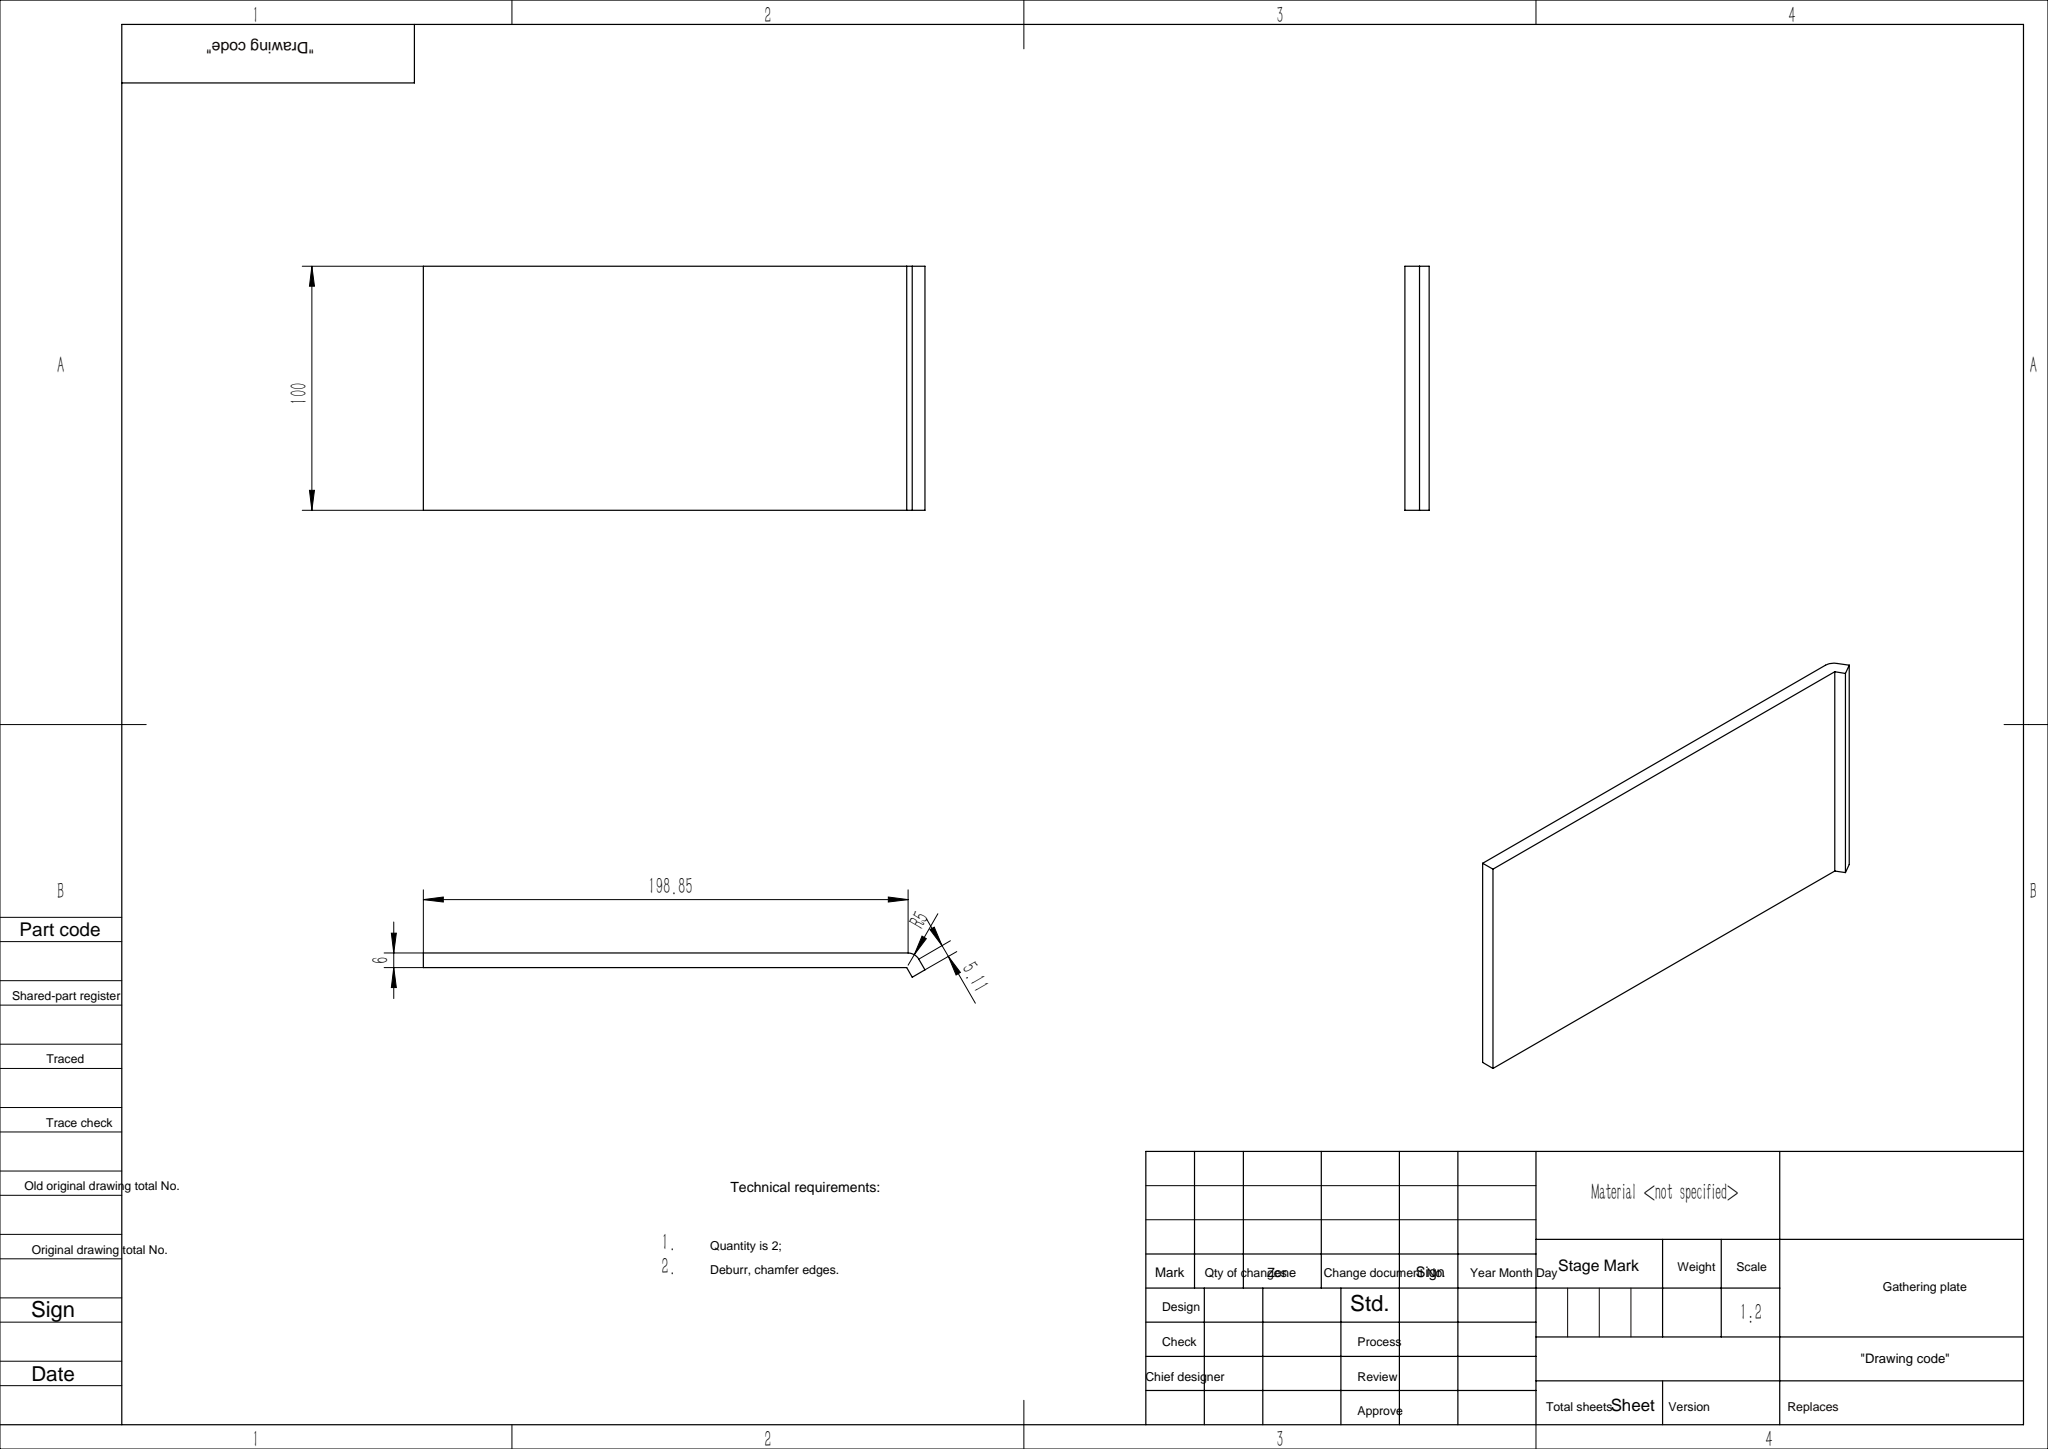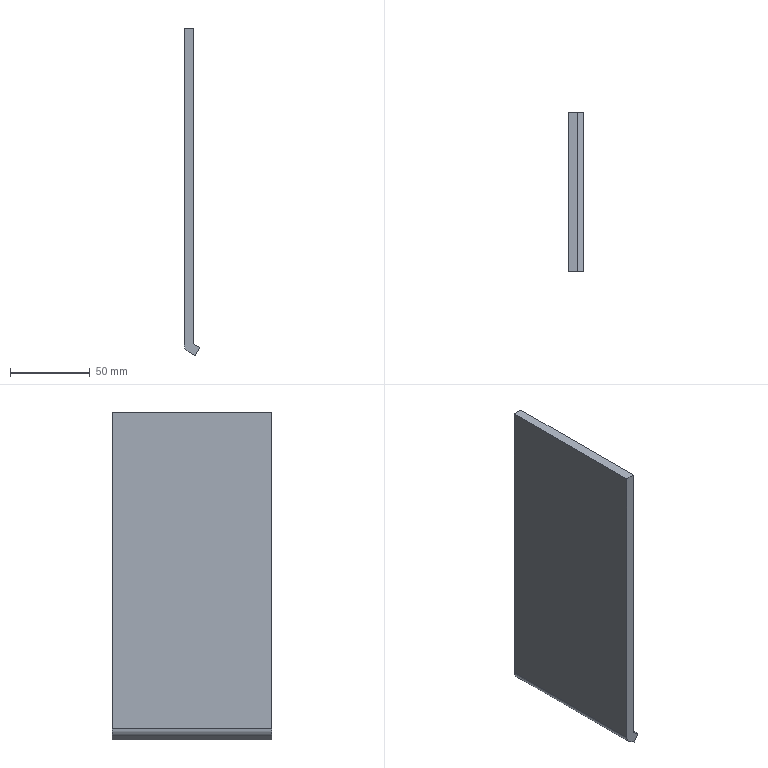Part | SolidWorks | features Extrusion 1, Fillet 1 | 1 solid | 9 faces | box 9.928 x 100 x 205.732 mm | volume 123626 mm3 | plane 8 | cylinder 1 | commonest cylinder face diameters 10 x1
STEP:
#1=CARTESIAN_POINT('',(-3.,0.,0.));
#2=VERTEX_POINT('',#1);
#3=CARTESIAN_POINT('',(3.,0.,0.));
#4=VERTEX_POINT('',#3);
#5=CARTESIAN_POINT('',(-3.,0.,0.));
#6=DIRECTION('',(1.,0.,0.));
#7=VECTOR('',#6,1000.);
#8=LINE('',#5,#7);
#9=EDGE_CURVE('',#2,#4,#8,.T.);
#10=ORIENTED_EDGE('',*,*,#9,.T.);
#11=CARTESIAN_POINT('',(3.,100.,0.));
#12=VERTEX_POINT('',#11);
#13=CARTESIAN_POINT('',(3.,100.,0.));
#14=DIRECTION('',(0.,-1.,0.));
#15=VECTOR('',#14,1000.);
#16=LINE('',#13,#15);
#17=EDGE_CURVE('',#12,#4,#16,.T.);
#18=ORIENTED_EDGE('',*,*,#17,.F.);
#19=CARTESIAN_POINT('',(-3.,100.,0.));
#20=VERTEX_POINT('',#19);
#21=CARTESIAN_POINT('',(-3.,100.,0.));
#22=DIRECTION('',(1.,0.,0.));
#23=VECTOR('',#22,1000.);
#24=LINE('',#21,#23);
#25=EDGE_CURVE('',#20,#12,#24,.T.);
#26=ORIENTED_EDGE('',*,*,#25,.F.);
#27=CARTESIAN_POINT('',(-3.,100.,0.));
#28=DIRECTION('',(0.,-1.,0.));
#29=VECTOR('',#28,1000.);
#30=LINE('',#27,#29);
#31=EDGE_CURVE('',#20,#2,#30,.T.);
#32=ORIENTED_EDGE('',*,*,#31,.T.);
#33=EDGE_LOOP('',(#10,#18,#26,#32));
#34=FACE_OUTER_BOUND('',#33,.T.);
#35=CARTESIAN_POINT('',(-3.,100.,0.));
#36=DIRECTION('',(0.,0.,-1.));
#37=DIRECTION('',(-1.,0.,0.));
#38=AXIS2_PLACEMENT_3D('',#35,#36,#37);
#39=PLANE('',#38);
#40=ADVANCED_FACE('',(#34),#39,.F.);
#41=CARTESIAN_POINT('',(3.,0.,-198.268));
#42=VERTEX_POINT('',#41);
#43=CARTESIAN_POINT('',(3.,0.,0.));
#44=DIRECTION('',(0.,0.,-1.));
#45=VECTOR('',#44,1000.);
#46=LINE('',#43,#45);
#47=EDGE_CURVE('',#4,#42,#46,.T.);
#48=ORIENTED_EDGE('',*,*,#47,.T.);
#49=CARTESIAN_POINT('',(3.,100.,-198.268));
#50=VERTEX_POINT('',#49);
#51=CARTESIAN_POINT('',(3.,100.,-198.268));
#52=DIRECTION('',(0.,-1.,0.));
#53=VECTOR('',#52,1000.);
#54=LINE('',#51,#53);
#55=EDGE_CURVE('',#50,#42,#54,.T.);
#56=ORIENTED_EDGE('',*,*,#55,.F.);
#57=CARTESIAN_POINT('',(3.,100.,0.));
#58=DIRECTION('',(0.,0.,-1.));
#59=VECTOR('',#58,1000.);
#60=LINE('',#57,#59);
#61=EDGE_CURVE('',#12,#50,#60,.T.);
#62=ORIENTED_EDGE('',*,*,#61,.F.);
#63=ORIENTED_EDGE('',*,*,#17,.T.);
#64=EDGE_LOOP('',(#48,#56,#62,#63));
#65=FACE_OUTER_BOUND('',#64,.T.);
#66=CARTESIAN_POINT('',(3.,100.,0.));
#67=DIRECTION('',(-1.,0.,0.));
#68=DIRECTION('',(0.,0.,1.));
#69=AXIS2_PLACEMENT_3D('',#66,#67,#68);
#70=PLANE('',#69);
#71=ADVANCED_FACE('',(#65),#70,.F.);
#72=CARTESIAN_POINT('',(6.928,0.,-200.536));
#73=VERTEX_POINT('',#72);
#74=CARTESIAN_POINT('',(3.,0.,-198.268));
#75=DIRECTION('',(0.866,0.,-0.5));
#76=VECTOR('',#75,1000.);
#77=LINE('',#74,#76);
#78=EDGE_CURVE('',#42,#73,#77,.T.);
#79=ORIENTED_EDGE('',*,*,#78,.T.);
#80=CARTESIAN_POINT('',(6.928,100.,-200.536));
#81=VERTEX_POINT('',#80);
#82=CARTESIAN_POINT('',(6.928,100.,-200.536));
#83=DIRECTION('',(0.,-1.,0.));
#84=VECTOR('',#83,1000.);
#85=LINE('',#82,#84);
#86=EDGE_CURVE('',#81,#73,#85,.T.);
#87=ORIENTED_EDGE('',*,*,#86,.F.);
#88=CARTESIAN_POINT('',(3.,100.,-198.268));
#89=DIRECTION('',(0.866,0.,-0.5));
#90=VECTOR('',#89,1000.);
#91=LINE('',#88,#90);
#92=EDGE_CURVE('',#50,#81,#91,.T.);
#93=ORIENTED_EDGE('',*,*,#92,.F.);
#94=ORIENTED_EDGE('',*,*,#55,.T.);
#95=EDGE_LOOP('',(#79,#87,#93,#94));
#96=FACE_OUTER_BOUND('',#95,.T.);
#97=CARTESIAN_POINT('',(3.,100.,-198.268));
#98=DIRECTION('',(-0.5,0.,-0.866));
#99=DIRECTION('',(-0.866,0.,0.5));
#100=AXIS2_PLACEMENT_3D('',#97,#98,#99);
#101=PLANE('',#100);
#102=ADVANCED_FACE('',(#96),#101,.F.);
#103=CARTESIAN_POINT('',(3.928,0.,-205.732));
#104=VERTEX_POINT('',#103);
#105=CARTESIAN_POINT('',(3.928,0.,-205.732));
#106=DIRECTION('',(-0.5,0.,-0.866));
#107=VECTOR('',#106,1000.);
#108=LINE('',#105,#107);
#109=EDGE_CURVE('',#73,#104,#108,.T.);
#110=ORIENTED_EDGE('',*,*,#109,.T.);
#111=CARTESIAN_POINT('',(3.928,100.,-205.732));
#112=VERTEX_POINT('',#111);
#113=CARTESIAN_POINT('',(3.928,100.,-205.732));
#114=DIRECTION('',(0.,-1.,0.));
#115=VECTOR('',#114,1000.);
#116=LINE('',#113,#115);
#117=EDGE_CURVE('',#112,#104,#116,.T.);
#118=ORIENTED_EDGE('',*,*,#117,.F.);
#119=CARTESIAN_POINT('',(3.928,100.,-205.732));
#120=DIRECTION('',(-0.5,0.,-0.866));
#121=VECTOR('',#120,1000.);
#122=LINE('',#119,#121);
#123=EDGE_CURVE('',#81,#112,#122,.T.);
#124=ORIENTED_EDGE('',*,*,#123,.F.);
#125=ORIENTED_EDGE('',*,*,#86,.T.);
#126=EDGE_LOOP('',(#110,#118,#124,#125));
#127=FACE_OUTER_BOUND('',#126,.T.);
#128=CARTESIAN_POINT('',(3.928,100.,-205.732));
#129=DIRECTION('',(-0.866,0.,0.5));
#130=DIRECTION('',(0.5,0.,0.866));
#131=AXIS2_PLACEMENT_3D('',#128,#129,#130);
#132=PLANE('',#131);
#133=ADVANCED_FACE('',(#127),#132,.F.);
#134=CARTESIAN_POINT('',(-0.5,0.,-203.175));
#135=VERTEX_POINT('',#134);
#136=CARTESIAN_POINT('',(-3.,0.,-201.732));
#137=DIRECTION('',(-0.866,0.,0.5));
#138=VECTOR('',#137,1000.);
#139=LINE('',#136,#138);
#140=EDGE_CURVE('',#104,#135,#139,.T.);
#141=ORIENTED_EDGE('',*,*,#140,.T.);
#142=CARTESIAN_POINT('',(-0.5,100.,-203.175));
#143=VERTEX_POINT('',#142);
#144=CARTESIAN_POINT('',(-0.5,100.,-203.175));
#145=DIRECTION('',(0.,1.,0.));
#146=VECTOR('',#145,1000.);
#147=LINE('',#144,#146);
#148=EDGE_CURVE('',#135,#143,#147,.T.);
#149=ORIENTED_EDGE('',*,*,#148,.T.);
#150=CARTESIAN_POINT('',(-3.,100.,-201.732));
#151=DIRECTION('',(-0.866,0.,0.5));
#152=VECTOR('',#151,1000.);
#153=LINE('',#150,#152);
#154=EDGE_CURVE('',#112,#143,#153,.T.);
#155=ORIENTED_EDGE('',*,*,#154,.F.);
#156=ORIENTED_EDGE('',*,*,#117,.T.);
#157=EDGE_LOOP('',(#141,#149,#155,#156));
#158=FACE_OUTER_BOUND('',#157,.T.);
#159=CARTESIAN_POINT('',(-3.,100.,-201.732));
#160=DIRECTION('',(0.5,0.,0.866));
#161=DIRECTION('',(0.866,0.,-0.5));
#162=AXIS2_PLACEMENT_3D('',#159,#160,#161);
#163=PLANE('',#162);
#164=ADVANCED_FACE('',(#158),#163,.F.);
#165=CARTESIAN_POINT('',(-3.,100.,-198.845));
#166=VERTEX_POINT('',#165);
#167=CARTESIAN_POINT('',(-3.,100.,0.));
#168=DIRECTION('',(0.,0.,1.));
#169=VECTOR('',#168,1000.);
#170=LINE('',#167,#169);
#171=EDGE_CURVE('',#166,#20,#170,.T.);
#172=ORIENTED_EDGE('',*,*,#171,.F.);
#173=CARTESIAN_POINT('',(-3.,0.,-198.845));
#174=VERTEX_POINT('',#173);
#175=CARTESIAN_POINT('',(-3.,100.,-198.845));
#176=DIRECTION('',(0.,-1.,0.));
#177=VECTOR('',#176,1000.);
#178=LINE('',#175,#177);
#179=EDGE_CURVE('',#166,#174,#178,.T.);
#180=ORIENTED_EDGE('',*,*,#179,.T.);
#181=CARTESIAN_POINT('',(-3.,0.,0.));
#182=DIRECTION('',(0.,0.,1.));
#183=VECTOR('',#182,1000.);
#184=LINE('',#181,#183);
#185=EDGE_CURVE('',#174,#2,#184,.T.);
#186=ORIENTED_EDGE('',*,*,#185,.T.);
#187=ORIENTED_EDGE('',*,*,#31,.F.);
#188=EDGE_LOOP('',(#172,#180,#186,#187));
#189=FACE_OUTER_BOUND('',#188,.T.);
#190=CARTESIAN_POINT('',(-3.,100.,0.));
#191=DIRECTION('',(1.,0.,0.));
#192=DIRECTION('',(0.,0.,-1.));
#193=AXIS2_PLACEMENT_3D('',#190,#191,#192);
#194=PLANE('',#193);
#195=ADVANCED_FACE('',(#189),#194,.F.);
#196=ORIENTED_EDGE('',*,*,#154,.T.);
#197=CARTESIAN_POINT('',(2.,100.,-198.845));
#198=DIRECTION('',(0.,1.,0.));
#199=DIRECTION('',(0.,0.,1.));
#200=AXIS2_PLACEMENT_3D('',#197,#198,#199);
#201=CIRCLE('',#200,5.);
#202=EDGE_CURVE('',#143,#166,#201,.T.);
#203=ORIENTED_EDGE('',*,*,#202,.T.);
#204=ORIENTED_EDGE('',*,*,#171,.T.);
#205=ORIENTED_EDGE('',*,*,#25,.T.);
#206=ORIENTED_EDGE('',*,*,#61,.T.);
#207=ORIENTED_EDGE('',*,*,#92,.T.);
#208=ORIENTED_EDGE('',*,*,#123,.T.);
#209=EDGE_LOOP('',(#196,#203,#204,#205,#206,#207,#208));
#210=FACE_OUTER_BOUND('',#209,.T.);
#211=CARTESIAN_POINT('',(0.,100.,0.));
#212=DIRECTION('',(0.,1.,0.));
#213=DIRECTION('',(0.,0.,1.));
#214=AXIS2_PLACEMENT_3D('',#211,#212,#213);
#215=PLANE('',#214);
#216=ADVANCED_FACE('',(#210),#215,.T.);
#217=ORIENTED_EDGE('',*,*,#185,.F.);
#218=CARTESIAN_POINT('',(2.,0.,-198.845));
#219=DIRECTION('',(0.,-1.,0.));
#220=DIRECTION('',(0.,0.,1.));
#221=AXIS2_PLACEMENT_3D('',#218,#219,#220);
#222=CIRCLE('',#221,5.);
#223=EDGE_CURVE('',#174,#135,#222,.T.);
#224=ORIENTED_EDGE('',*,*,#223,.T.);
#225=ORIENTED_EDGE('',*,*,#140,.F.);
#226=ORIENTED_EDGE('',*,*,#109,.F.);
#227=ORIENTED_EDGE('',*,*,#78,.F.);
#228=ORIENTED_EDGE('',*,*,#47,.F.);
#229=ORIENTED_EDGE('',*,*,#9,.F.);
#230=EDGE_LOOP('',(#217,#224,#225,#226,#227,#228,#229));
#231=FACE_OUTER_BOUND('',#230,.T.);
#232=CARTESIAN_POINT('',(0.,0.,0.));
#233=DIRECTION('',(0.,1.,0.));
#234=DIRECTION('',(0.,0.,1.));
#235=AXIS2_PLACEMENT_3D('',#232,#233,#234);
#236=PLANE('',#235);
#237=ADVANCED_FACE('',(#231),#236,.F.);
#238=ORIENTED_EDGE('',*,*,#202,.F.);
#239=ORIENTED_EDGE('',*,*,#148,.F.);
#240=ORIENTED_EDGE('',*,*,#223,.F.);
#241=ORIENTED_EDGE('',*,*,#179,.F.);
#242=EDGE_LOOP('',(#238,#239,#240,#241));
#243=FACE_OUTER_BOUND('',#242,.T.);
#244=CARTESIAN_POINT('',(2.,100.,-198.845));
#245=DIRECTION('',(0.,-1.,0.));
#246=DIRECTION('',(0.,0.,-1.));
#247=AXIS2_PLACEMENT_3D('',#244,#245,#246);
#248=CYLINDRICAL_SURFACE('',#247,5.);
#249=ADVANCED_FACE('',(#243),#248,.T.);
#250=CLOSED_SHELL('',(#40,#71,#102,#133,#164,#195,#216,#237,#249));
#251=MANIFOLD_SOLID_BREP('',#250);
#252=CARTESIAN_POINT('',(0.,0.,0.));
#253=DIRECTION('',(0.,0.,1.));
#254=DIRECTION('',(1.,0.,0.));
#255=AXIS2_PLACEMENT_3D('',#252,#253,#254);
#256=(LENGTH_UNIT()NAMED_UNIT(*)SI_UNIT(.MILLI.,.METRE.));
#257=UNCERTAINTY_MEASURE_WITH_UNIT(LENGTH_MEASURE(0.00001),#256,'','');
#258=(NAMED_UNIT(*)PLANE_ANGLE_UNIT()SI_UNIT($,.RADIAN.));
#259=(NAMED_UNIT(*)SI_UNIT($,.STERADIAN.)SOLID_ANGLE_UNIT());
#260=(GEOMETRIC_REPRESENTATION_CONTEXT(3)GLOBAL_UNCERTAINTY_ASSIGNED_CONTEXT((#257))GLOBAL_UNIT_ASSIGNED_CONTEXT((#256,#258,#259))REPRESENTATION_CONTEXT('',''));
#261=ADVANCED_BREP_SHAPE_REPRESENTATION('',(#251,#255),#260);